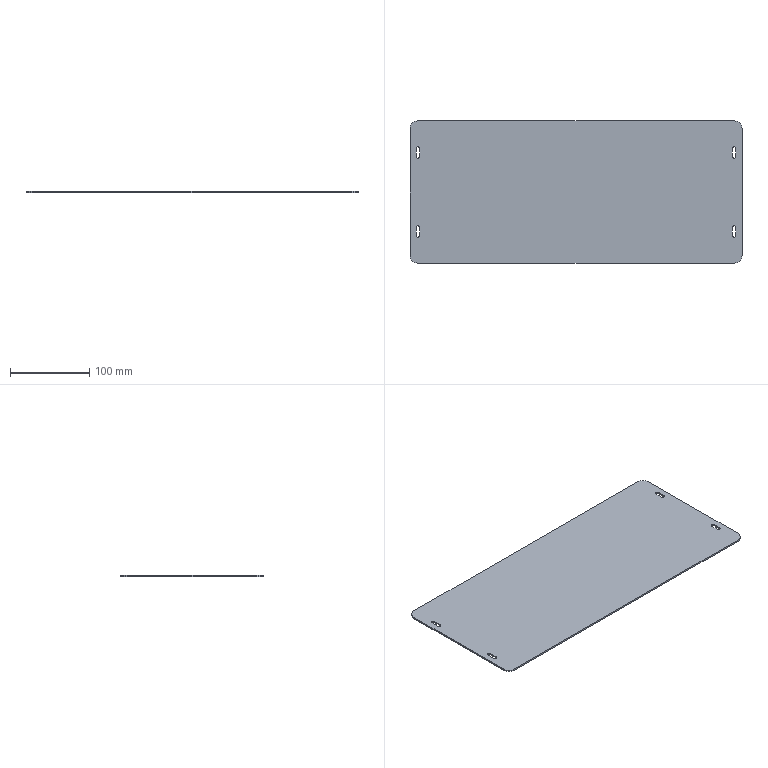Part | SolidWorks | features RefAxis 2, Extrusion 1, Fillet 1, HoleWzd 1, ICE 1 | 1 solid | 26 faces | box 420 x 180 x 2 mm | volume 150541 mm3 | plane 14 | cylinder 12 | commonest cylinder face diameters 4.5 x8 20 x4
STEP:
#1=CARTESIAN_POINT('',(210.,-80.,2.));
#2=VERTEX_POINT('',#1);
#3=CARTESIAN_POINT('',(210.,80.,2.));
#4=VERTEX_POINT('',#3);
#5=CARTESIAN_POINT('',(210.,90.,2.));
#6=DIRECTION('',(0.,1.,0.));
#7=VECTOR('',#6,1000.);
#8=LINE('',#5,#7);
#9=EDGE_CURVE('',#2,#4,#8,.T.);
#10=ORIENTED_EDGE('',*,*,#9,.F.);
#11=CARTESIAN_POINT('',(210.,-80.,0.));
#12=VERTEX_POINT('',#11);
#13=CARTESIAN_POINT('',(210.,-80.,2.));
#14=DIRECTION('',(0.,0.,-1.));
#15=VECTOR('',#14,1000.);
#16=LINE('',#13,#15);
#17=EDGE_CURVE('',#2,#12,#16,.T.);
#18=ORIENTED_EDGE('',*,*,#17,.T.);
#19=CARTESIAN_POINT('',(210.,80.,0.));
#20=VERTEX_POINT('',#19);
#21=CARTESIAN_POINT('',(210.,90.,0.));
#22=DIRECTION('',(0.,1.,0.));
#23=VECTOR('',#22,1000.);
#24=LINE('',#21,#23);
#25=EDGE_CURVE('',#12,#20,#24,.T.);
#26=ORIENTED_EDGE('',*,*,#25,.T.);
#27=CARTESIAN_POINT('',(210.,80.,2.));
#28=DIRECTION('',(0.,0.,1.));
#29=VECTOR('',#28,1000.);
#30=LINE('',#27,#29);
#31=EDGE_CURVE('',#20,#4,#30,.T.);
#32=ORIENTED_EDGE('',*,*,#31,.T.);
#33=EDGE_LOOP('',(#10,#18,#26,#32));
#34=FACE_OUTER_BOUND('',#33,.T.);
#35=CARTESIAN_POINT('',(210.,90.,2.));
#36=DIRECTION('',(-1.,0.,0.));
#37=DIRECTION('',(0.,0.,1.));
#38=AXIS2_PLACEMENT_3D('',#35,#36,#37);
#39=PLANE('',#38);
#40=ADVANCED_FACE('',(#34),#39,.F.);
#41=CARTESIAN_POINT('',(200.,90.,0.));
#42=VERTEX_POINT('',#41);
#43=CARTESIAN_POINT('',(-200.,90.,0.));
#44=VERTEX_POINT('',#43);
#45=CARTESIAN_POINT('',(-210.,90.,0.));
#46=DIRECTION('',(-1.,0.,0.));
#47=VECTOR('',#46,1000.);
#48=LINE('',#45,#47);
#49=EDGE_CURVE('',#42,#44,#48,.T.);
#50=ORIENTED_EDGE('',*,*,#49,.T.);
#51=CARTESIAN_POINT('',(-200.,90.,2.));
#52=VERTEX_POINT('',#51);
#53=CARTESIAN_POINT('',(-200.,90.,2.));
#54=DIRECTION('',(0.,0.,1.));
#55=VECTOR('',#54,1000.);
#56=LINE('',#53,#55);
#57=EDGE_CURVE('',#44,#52,#56,.T.);
#58=ORIENTED_EDGE('',*,*,#57,.T.);
#59=CARTESIAN_POINT('',(200.,90.,2.));
#60=VERTEX_POINT('',#59);
#61=CARTESIAN_POINT('',(-210.,90.,2.));
#62=DIRECTION('',(-1.,0.,0.));
#63=VECTOR('',#62,1000.);
#64=LINE('',#61,#63);
#65=EDGE_CURVE('',#60,#52,#64,.T.);
#66=ORIENTED_EDGE('',*,*,#65,.F.);
#67=CARTESIAN_POINT('',(200.,90.,2.));
#68=DIRECTION('',(0.,0.,-1.));
#69=VECTOR('',#68,1000.);
#70=LINE('',#67,#69);
#71=EDGE_CURVE('',#60,#42,#70,.T.);
#72=ORIENTED_EDGE('',*,*,#71,.T.);
#73=EDGE_LOOP('',(#50,#58,#66,#72));
#74=FACE_OUTER_BOUND('',#73,.T.);
#75=CARTESIAN_POINT('',(-210.,90.,2.));
#76=DIRECTION('',(0.,-1.,0.));
#77=DIRECTION('',(0.,0.,-1.));
#78=AXIS2_PLACEMENT_3D('',#75,#76,#77);
#79=PLANE('',#78);
#80=ADVANCED_FACE('',(#74),#79,.F.);
#81=CARTESIAN_POINT('',(-210.,80.,0.));
#82=VERTEX_POINT('',#81);
#83=CARTESIAN_POINT('',(-210.,-80.,0.));
#84=VERTEX_POINT('',#83);
#85=CARTESIAN_POINT('',(-210.,90.,0.));
#86=DIRECTION('',(0.,-1.,0.));
#87=VECTOR('',#86,1000.);
#88=LINE('',#85,#87);
#89=EDGE_CURVE('',#82,#84,#88,.T.);
#90=ORIENTED_EDGE('',*,*,#89,.T.);
#91=CARTESIAN_POINT('',(-210.,-80.,2.));
#92=VERTEX_POINT('',#91);
#93=CARTESIAN_POINT('',(-210.,-80.,2.));
#94=DIRECTION('',(0.,0.,1.));
#95=VECTOR('',#94,1000.);
#96=LINE('',#93,#95);
#97=EDGE_CURVE('',#84,#92,#96,.T.);
#98=ORIENTED_EDGE('',*,*,#97,.T.);
#99=CARTESIAN_POINT('',(-210.,80.,2.));
#100=VERTEX_POINT('',#99);
#101=CARTESIAN_POINT('',(-210.,90.,2.));
#102=DIRECTION('',(0.,-1.,0.));
#103=VECTOR('',#102,1000.);
#104=LINE('',#101,#103);
#105=EDGE_CURVE('',#100,#92,#104,.T.);
#106=ORIENTED_EDGE('',*,*,#105,.F.);
#107=CARTESIAN_POINT('',(-210.,80.,2.));
#108=DIRECTION('',(0.,0.,-1.));
#109=VECTOR('',#108,1000.);
#110=LINE('',#107,#109);
#111=EDGE_CURVE('',#100,#82,#110,.T.);
#112=ORIENTED_EDGE('',*,*,#111,.T.);
#113=EDGE_LOOP('',(#90,#98,#106,#112));
#114=FACE_OUTER_BOUND('',#113,.T.);
#115=CARTESIAN_POINT('',(-210.,90.,2.));
#116=DIRECTION('',(1.,0.,0.));
#117=DIRECTION('',(0.,0.,-1.));
#118=AXIS2_PLACEMENT_3D('',#115,#116,#117);
#119=PLANE('',#118);
#120=ADVANCED_FACE('',(#114),#119,.F.);
#121=CARTESIAN_POINT('',(-200.,-90.,2.));
#122=VERTEX_POINT('',#121);
#123=CARTESIAN_POINT('',(200.,-90.,2.));
#124=VERTEX_POINT('',#123);
#125=CARTESIAN_POINT('',(-210.,-90.,2.));
#126=DIRECTION('',(1.,0.,0.));
#127=VECTOR('',#126,1000.);
#128=LINE('',#125,#127);
#129=EDGE_CURVE('',#122,#124,#128,.T.);
#130=ORIENTED_EDGE('',*,*,#129,.F.);
#131=CARTESIAN_POINT('',(-200.,-90.,0.));
#132=VERTEX_POINT('',#131);
#133=CARTESIAN_POINT('',(-200.,-90.,2.));
#134=DIRECTION('',(0.,0.,-1.));
#135=VECTOR('',#134,1000.);
#136=LINE('',#133,#135);
#137=EDGE_CURVE('',#122,#132,#136,.T.);
#138=ORIENTED_EDGE('',*,*,#137,.T.);
#139=CARTESIAN_POINT('',(200.,-90.,0.));
#140=VERTEX_POINT('',#139);
#141=CARTESIAN_POINT('',(-210.,-90.,0.));
#142=DIRECTION('',(1.,0.,0.));
#143=VECTOR('',#142,1000.);
#144=LINE('',#141,#143);
#145=EDGE_CURVE('',#132,#140,#144,.T.);
#146=ORIENTED_EDGE('',*,*,#145,.T.);
#147=CARTESIAN_POINT('',(200.,-90.,2.));
#148=DIRECTION('',(0.,0.,1.));
#149=VECTOR('',#148,1000.);
#150=LINE('',#147,#149);
#151=EDGE_CURVE('',#140,#124,#150,.T.);
#152=ORIENTED_EDGE('',*,*,#151,.T.);
#153=EDGE_LOOP('',(#130,#138,#146,#152));
#154=FACE_OUTER_BOUND('',#153,.T.);
#155=CARTESIAN_POINT('',(-210.,-90.,2.));
#156=DIRECTION('',(0.,1.,0.));
#157=DIRECTION('',(0.,0.,1.));
#158=AXIS2_PLACEMENT_3D('',#155,#156,#157);
#159=PLANE('',#158);
#160=ADVANCED_FACE('',(#154),#159,.F.);
#161=CARTESIAN_POINT('',(-197.75,55.,2.));
#162=VERTEX_POINT('',#161);
#163=CARTESIAN_POINT('',(-202.25,55.,2.));
#164=VERTEX_POINT('',#163);
#165=CARTESIAN_POINT('',(-200.,55.,2.));
#166=DIRECTION('',(0.,0.,1.));
#167=DIRECTION('',(-1.,0.,0.));
#168=AXIS2_PLACEMENT_3D('',#165,#166,#167);
#169=CIRCLE('',#168,2.25);
#170=EDGE_CURVE('',#162,#164,#169,.T.);
#171=ORIENTED_EDGE('',*,*,#170,.F.);
#172=CARTESIAN_POINT('',(-197.75,45.,2.));
#173=VERTEX_POINT('',#172);
#174=CARTESIAN_POINT('',(-197.75,55.,2.));
#175=DIRECTION('',(0.,1.,0.));
#176=VECTOR('',#175,1000.);
#177=LINE('',#174,#176);
#178=EDGE_CURVE('',#173,#162,#177,.T.);
#179=ORIENTED_EDGE('',*,*,#178,.F.);
#180=CARTESIAN_POINT('',(-202.25,45.,2.));
#181=VERTEX_POINT('',#180);
#182=CARTESIAN_POINT('',(-200.,45.,2.));
#183=DIRECTION('',(0.,0.,1.));
#184=DIRECTION('',(-1.,0.,0.));
#185=AXIS2_PLACEMENT_3D('',#182,#183,#184);
#186=CIRCLE('',#185,2.25);
#187=EDGE_CURVE('',#181,#173,#186,.T.);
#188=ORIENTED_EDGE('',*,*,#187,.F.);
#189=CARTESIAN_POINT('',(-202.25,55.,2.));
#190=DIRECTION('',(0.,-1.,0.));
#191=VECTOR('',#190,1000.);
#192=LINE('',#189,#191);
#193=EDGE_CURVE('',#164,#181,#192,.T.);
#194=ORIENTED_EDGE('',*,*,#193,.F.);
#195=EDGE_LOOP('',(#171,#179,#188,#194));
#196=FACE_BOUND('',#195,.T.);
#197=CARTESIAN_POINT('',(-202.25,-55.,2.));
#198=VERTEX_POINT('',#197);
#199=CARTESIAN_POINT('',(-197.75,-55.,2.));
#200=VERTEX_POINT('',#199);
#201=CARTESIAN_POINT('',(-200.,-55.,2.));
#202=DIRECTION('',(0.,0.,1.));
#203=DIRECTION('',(-1.,0.,0.));
#204=AXIS2_PLACEMENT_3D('',#201,#202,#203);
#205=CIRCLE('',#204,2.25);
#206=EDGE_CURVE('',#198,#200,#205,.T.);
#207=ORIENTED_EDGE('',*,*,#206,.F.);
#208=CARTESIAN_POINT('',(-202.25,-45.,2.));
#209=VERTEX_POINT('',#208);
#210=CARTESIAN_POINT('',(-202.25,-55.,2.));
#211=DIRECTION('',(0.,-1.,0.));
#212=VECTOR('',#211,1000.);
#213=LINE('',#210,#212);
#214=EDGE_CURVE('',#209,#198,#213,.T.);
#215=ORIENTED_EDGE('',*,*,#214,.F.);
#216=CARTESIAN_POINT('',(-197.75,-45.,2.));
#217=VERTEX_POINT('',#216);
#218=CARTESIAN_POINT('',(-200.,-45.,2.));
#219=DIRECTION('',(0.,0.,1.));
#220=DIRECTION('',(-1.,0.,0.));
#221=AXIS2_PLACEMENT_3D('',#218,#219,#220);
#222=CIRCLE('',#221,2.25);
#223=EDGE_CURVE('',#217,#209,#222,.T.);
#224=ORIENTED_EDGE('',*,*,#223,.F.);
#225=CARTESIAN_POINT('',(-197.75,-55.,2.));
#226=DIRECTION('',(0.,1.,0.));
#227=VECTOR('',#226,1000.);
#228=LINE('',#225,#227);
#229=EDGE_CURVE('',#200,#217,#228,.T.);
#230=ORIENTED_EDGE('',*,*,#229,.F.);
#231=EDGE_LOOP('',(#207,#215,#224,#230));
#232=FACE_BOUND('',#231,.T.);
#233=CARTESIAN_POINT('',(197.75,-55.,2.));
#234=VERTEX_POINT('',#233);
#235=CARTESIAN_POINT('',(202.25,-55.,2.));
#236=VERTEX_POINT('',#235);
#237=CARTESIAN_POINT('',(200.,-55.,2.));
#238=DIRECTION('',(0.,0.,1.));
#239=DIRECTION('',(1.,0.,0.));
#240=AXIS2_PLACEMENT_3D('',#237,#238,#239);
#241=CIRCLE('',#240,2.25);
#242=EDGE_CURVE('',#234,#236,#241,.T.);
#243=ORIENTED_EDGE('',*,*,#242,.F.);
#244=CARTESIAN_POINT('',(197.75,-45.,2.));
#245=VERTEX_POINT('',#244);
#246=CARTESIAN_POINT('',(197.75,-55.,2.));
#247=DIRECTION('',(0.,-1.,0.));
#248=VECTOR('',#247,1000.);
#249=LINE('',#246,#248);
#250=EDGE_CURVE('',#245,#234,#249,.T.);
#251=ORIENTED_EDGE('',*,*,#250,.F.);
#252=CARTESIAN_POINT('',(202.25,-45.,2.));
#253=VERTEX_POINT('',#252);
#254=CARTESIAN_POINT('',(200.,-45.,2.));
#255=DIRECTION('',(0.,0.,1.));
#256=DIRECTION('',(1.,0.,0.));
#257=AXIS2_PLACEMENT_3D('',#254,#255,#256);
#258=CIRCLE('',#257,2.25);
#259=EDGE_CURVE('',#253,#245,#258,.T.);
#260=ORIENTED_EDGE('',*,*,#259,.F.);
#261=CARTESIAN_POINT('',(202.25,-55.,2.));
#262=DIRECTION('',(0.,1.,0.));
#263=VECTOR('',#262,1000.);
#264=LINE('',#261,#263);
#265=EDGE_CURVE('',#236,#253,#264,.T.);
#266=ORIENTED_EDGE('',*,*,#265,.F.);
#267=EDGE_LOOP('',(#243,#251,#260,#266));
#268=FACE_BOUND('',#267,.T.);
#269=CARTESIAN_POINT('',(202.25,55.,2.));
#270=VERTEX_POINT('',#269);
#271=CARTESIAN_POINT('',(197.75,55.,2.));
#272=VERTEX_POINT('',#271);
#273=CARTESIAN_POINT('',(200.,55.,2.));
#274=DIRECTION('',(0.,0.,1.));
#275=DIRECTION('',(1.,0.,0.));
#276=AXIS2_PLACEMENT_3D('',#273,#274,#275);
#277=CIRCLE('',#276,2.25);
#278=EDGE_CURVE('',#270,#272,#277,.T.);
#279=ORIENTED_EDGE('',*,*,#278,.F.);
#280=CARTESIAN_POINT('',(202.25,45.,2.));
#281=VERTEX_POINT('',#280);
#282=CARTESIAN_POINT('',(202.25,55.,2.));
#283=DIRECTION('',(0.,1.,0.));
#284=VECTOR('',#283,1000.);
#285=LINE('',#282,#284);
#286=EDGE_CURVE('',#281,#270,#285,.T.);
#287=ORIENTED_EDGE('',*,*,#286,.F.);
#288=CARTESIAN_POINT('',(197.75,45.,2.));
#289=VERTEX_POINT('',#288);
#290=CARTESIAN_POINT('',(200.,45.,2.));
#291=DIRECTION('',(0.,0.,1.));
#292=DIRECTION('',(1.,0.,0.));
#293=AXIS2_PLACEMENT_3D('',#290,#291,#292);
#294=CIRCLE('',#293,2.25);
#295=EDGE_CURVE('',#289,#281,#294,.T.);
#296=ORIENTED_EDGE('',*,*,#295,.F.);
#297=CARTESIAN_POINT('',(197.75,55.,2.));
#298=DIRECTION('',(0.,-1.,0.));
#299=VECTOR('',#298,1000.);
#300=LINE('',#297,#299);
#301=EDGE_CURVE('',#272,#289,#300,.T.);
#302=ORIENTED_EDGE('',*,*,#301,.F.);
#303=EDGE_LOOP('',(#279,#287,#296,#302));
#304=FACE_BOUND('',#303,.T.);
#305=ORIENTED_EDGE('',*,*,#105,.T.);
#306=CARTESIAN_POINT('',(-200.,-80.,2.));
#307=DIRECTION('',(0.,0.,1.));
#308=DIRECTION('',(1.,0.,0.));
#309=AXIS2_PLACEMENT_3D('',#306,#307,#308);
#310=CIRCLE('',#309,10.);
#311=EDGE_CURVE('',#92,#122,#310,.T.);
#312=ORIENTED_EDGE('',*,*,#311,.T.);
#313=ORIENTED_EDGE('',*,*,#129,.T.);
#314=CARTESIAN_POINT('',(200.,-80.,2.));
#315=DIRECTION('',(0.,0.,1.));
#316=DIRECTION('',(1.,0.,0.));
#317=AXIS2_PLACEMENT_3D('',#314,#315,#316);
#318=CIRCLE('',#317,10.);
#319=EDGE_CURVE('',#124,#2,#318,.T.);
#320=ORIENTED_EDGE('',*,*,#319,.T.);
#321=ORIENTED_EDGE('',*,*,#9,.T.);
#322=CARTESIAN_POINT('',(200.,80.,2.));
#323=DIRECTION('',(0.,0.,1.));
#324=DIRECTION('',(1.,0.,0.));
#325=AXIS2_PLACEMENT_3D('',#322,#323,#324);
#326=CIRCLE('',#325,10.);
#327=EDGE_CURVE('',#4,#60,#326,.T.);
#328=ORIENTED_EDGE('',*,*,#327,.T.);
#329=ORIENTED_EDGE('',*,*,#65,.T.);
#330=CARTESIAN_POINT('',(-200.,80.,2.));
#331=DIRECTION('',(0.,0.,1.));
#332=DIRECTION('',(1.,0.,0.));
#333=AXIS2_PLACEMENT_3D('',#330,#331,#332);
#334=CIRCLE('',#333,10.);
#335=EDGE_CURVE('',#52,#100,#334,.T.);
#336=ORIENTED_EDGE('',*,*,#335,.T.);
#337=EDGE_LOOP('',(#305,#312,#313,#320,#321,#328,#329,#336));
#338=FACE_OUTER_BOUND('',#337,.T.);
#339=CARTESIAN_POINT('',(0.,0.,2.));
#340=DIRECTION('',(0.,0.,1.));
#341=DIRECTION('',(1.,0.,0.));
#342=AXIS2_PLACEMENT_3D('',#339,#340,#341);
#343=PLANE('',#342);
#344=ADVANCED_FACE('',(#196,#232,#268,#304,#338),#343,.T.);
#345=CARTESIAN_POINT('',(-197.75,45.,0.));
#346=VERTEX_POINT('',#345);
#347=CARTESIAN_POINT('',(-197.75,55.,0.));
#348=VERTEX_POINT('',#347);
#349=CARTESIAN_POINT('',(-197.75,0.,0.));
#350=DIRECTION('',(0.,1.,0.));
#351=VECTOR('',#350,1000.);
#352=LINE('',#349,#351);
#353=EDGE_CURVE('',#346,#348,#352,.T.);
#354=ORIENTED_EDGE('',*,*,#353,.T.);
#355=CARTESIAN_POINT('',(-202.25,55.,0.));
#356=VERTEX_POINT('',#355);
#357=CARTESIAN_POINT('',(-200.,55.,0.));
#358=DIRECTION('',(0.,0.,1.));
#359=DIRECTION('',(1.,0.,0.));
#360=AXIS2_PLACEMENT_3D('',#357,#358,#359);
#361=CIRCLE('',#360,2.25);
#362=EDGE_CURVE('',#348,#356,#361,.T.);
#363=ORIENTED_EDGE('',*,*,#362,.T.);
#364=CARTESIAN_POINT('',(-202.25,45.,0.));
#365=VERTEX_POINT('',#364);
#366=CARTESIAN_POINT('',(-202.25,0.,0.));
#367=DIRECTION('',(0.,-1.,0.));
#368=VECTOR('',#367,1000.);
#369=LINE('',#366,#368);
#370=EDGE_CURVE('',#356,#365,#369,.T.);
#371=ORIENTED_EDGE('',*,*,#370,.T.);
#372=CARTESIAN_POINT('',(-200.,45.,0.));
#373=DIRECTION('',(0.,0.,1.));
#374=DIRECTION('',(1.,0.,0.));
#375=AXIS2_PLACEMENT_3D('',#372,#373,#374);
#376=CIRCLE('',#375,2.25);
#377=EDGE_CURVE('',#365,#346,#376,.T.);
#378=ORIENTED_EDGE('',*,*,#377,.T.);
#379=EDGE_LOOP('',(#354,#363,#371,#378));
#380=FACE_BOUND('',#379,.T.);
#381=CARTESIAN_POINT('',(-202.25,-45.,0.));
#382=VERTEX_POINT('',#381);
#383=CARTESIAN_POINT('',(-202.25,-55.,0.));
#384=VERTEX_POINT('',#383);
#385=CARTESIAN_POINT('',(-202.25,0.,0.));
#386=DIRECTION('',(0.,-1.,0.));
#387=VECTOR('',#386,1000.);
#388=LINE('',#385,#387);
#389=EDGE_CURVE('',#382,#384,#388,.T.);
#390=ORIENTED_EDGE('',*,*,#389,.T.);
#391=CARTESIAN_POINT('',(-197.75,-55.,0.));
#392=VERTEX_POINT('',#391);
#393=CARTESIAN_POINT('',(-200.,-55.,0.));
#394=DIRECTION('',(0.,0.,1.));
#395=DIRECTION('',(1.,0.,0.));
#396=AXIS2_PLACEMENT_3D('',#393,#394,#395);
#397=CIRCLE('',#396,2.25);
#398=EDGE_CURVE('',#384,#392,#397,.T.);
#399=ORIENTED_EDGE('',*,*,#398,.T.);
#400=CARTESIAN_POINT('',(-197.75,-45.,0.));
#401=VERTEX_POINT('',#400);
#402=CARTESIAN_POINT('',(-197.75,0.,0.));
#403=DIRECTION('',(0.,1.,0.));
#404=VECTOR('',#403,1000.);
#405=LINE('',#402,#404);
#406=EDGE_CURVE('',#392,#401,#405,.T.);
#407=ORIENTED_EDGE('',*,*,#406,.T.);
#408=CARTESIAN_POINT('',(-200.,-45.,0.));
#409=DIRECTION('',(0.,0.,1.));
#410=DIRECTION('',(1.,0.,0.));
#411=AXIS2_PLACEMENT_3D('',#408,#409,#410);
#412=CIRCLE('',#411,2.25);
#413=EDGE_CURVE('',#401,#382,#412,.T.);
#414=ORIENTED_EDGE('',*,*,#413,.T.);
#415=EDGE_LOOP('',(#390,#399,#407,#414));
#416=FACE_BOUND('',#415,.T.);
#417=CARTESIAN_POINT('',(197.75,-45.,0.));
#418=VERTEX_POINT('',#417);
#419=CARTESIAN_POINT('',(197.75,-55.,0.));
#420=VERTEX_POINT('',#419);
#421=CARTESIAN_POINT('',(197.75,0.,0.));
#422=DIRECTION('',(0.,-1.,0.));
#423=VECTOR('',#422,1000.);
#424=LINE('',#421,#423);
#425=EDGE_CURVE('',#418,#420,#424,.T.);
#426=ORIENTED_EDGE('',*,*,#425,.T.);
#427=CARTESIAN_POINT('',(202.25,-55.,0.));
#428=VERTEX_POINT('',#427);
#429=CARTESIAN_POINT('',(200.,-55.,0.));
#430=DIRECTION('',(0.,0.,1.));
#431=DIRECTION('',(1.,0.,0.));
#432=AXIS2_PLACEMENT_3D('',#429,#430,#431);
#433=CIRCLE('',#432,2.25);
#434=EDGE_CURVE('',#420,#428,#433,.T.);
#435=ORIENTED_EDGE('',*,*,#434,.T.);
#436=CARTESIAN_POINT('',(202.25,-45.,0.));
#437=VERTEX_POINT('',#436);
#438=CARTESIAN_POINT('',(202.25,0.,0.));
#439=DIRECTION('',(0.,1.,0.));
#440=VECTOR('',#439,1000.);
#441=LINE('',#438,#440);
#442=EDGE_CURVE('',#428,#437,#441,.T.);
#443=ORIENTED_EDGE('',*,*,#442,.T.);
#444=CARTESIAN_POINT('',(200.,-45.,0.));
#445=DIRECTION('',(0.,0.,1.));
#446=DIRECTION('',(1.,0.,0.));
#447=AXIS2_PLACEMENT_3D('',#444,#445,#446);
#448=CIRCLE('',#447,2.25);
#449=EDGE_CURVE('',#437,#418,#448,.T.);
#450=ORIENTED_EDGE('',*,*,#449,.T.);
#451=EDGE_LOOP('',(#426,#435,#443,#450));
#452=FACE_BOUND('',#451,.T.);
#453=CARTESIAN_POINT('',(202.25,45.,0.));
#454=VERTEX_POINT('',#453);
#455=CARTESIAN_POINT('',(202.25,55.,0.));
#456=VERTEX_POINT('',#455);
#457=CARTESIAN_POINT('',(202.25,0.,0.));
#458=DIRECTION('',(0.,1.,0.));
#459=VECTOR('',#458,1000.);
#460=LINE('',#457,#459);
#461=EDGE_CURVE('',#454,#456,#460,.T.);
#462=ORIENTED_EDGE('',*,*,#461,.T.);
#463=CARTESIAN_POINT('',(197.75,55.,0.));
#464=VERTEX_POINT('',#463);
#465=CARTESIAN_POINT('',(200.,55.,0.));
#466=DIRECTION('',(0.,0.,1.));
#467=DIRECTION('',(1.,0.,0.));
#468=AXIS2_PLACEMENT_3D('',#465,#466,#467);
#469=CIRCLE('',#468,2.25);
#470=EDGE_CURVE('',#456,#464,#469,.T.);
#471=ORIENTED_EDGE('',*,*,#470,.T.);
#472=CARTESIAN_POINT('',(197.75,45.,0.));
#473=VERTEX_POINT('',#472);
#474=CARTESIAN_POINT('',(197.75,0.,0.));
#475=DIRECTION('',(0.,-1.,0.));
#476=VECTOR('',#475,1000.);
#477=LINE('',#474,#476);
#478=EDGE_CURVE('',#464,#473,#477,.T.);
#479=ORIENTED_EDGE('',*,*,#478,.T.);
#480=CARTESIAN_POINT('',(200.,45.,0.));
#481=DIRECTION('',(0.,0.,1.));
#482=DIRECTION('',(1.,0.,0.));
#483=AXIS2_PLACEMENT_3D('',#480,#481,#482);
#484=CIRCLE('',#483,2.25);
#485=EDGE_CURVE('',#473,#454,#484,.T.);
#486=ORIENTED_EDGE('',*,*,#485,.T.);
#487=EDGE_LOOP('',(#462,#471,#479,#486));
#488=FACE_BOUND('',#487,.T.);
#489=ORIENTED_EDGE('',*,*,#145,.F.);
#490=CARTESIAN_POINT('',(-200.,-80.,0.));
#491=DIRECTION('',(0.,0.,-1.));
#492=DIRECTION('',(1.,0.,0.));
#493=AXIS2_PLACEMENT_3D('',#490,#491,#492);
#494=CIRCLE('',#493,10.);
#495=EDGE_CURVE('',#132,#84,#494,.T.);
#496=ORIENTED_EDGE('',*,*,#495,.T.);
#497=ORIENTED_EDGE('',*,*,#89,.F.);
#498=CARTESIAN_POINT('',(-200.,80.,0.));
#499=DIRECTION('',(0.,0.,-1.));
#500=DIRECTION('',(1.,0.,0.));
#501=AXIS2_PLACEMENT_3D('',#498,#499,#500);
#502=CIRCLE('',#501,10.);
#503=EDGE_CURVE('',#82,#44,#502,.T.);
#504=ORIENTED_EDGE('',*,*,#503,.T.);
#505=ORIENTED_EDGE('',*,*,#49,.F.);
#506=CARTESIAN_POINT('',(200.,80.,0.));
#507=DIRECTION('',(0.,0.,-1.));
#508=DIRECTION('',(1.,0.,0.));
#509=AXIS2_PLACEMENT_3D('',#506,#507,#508);
#510=CIRCLE('',#509,10.);
#511=EDGE_CURVE('',#42,#20,#510,.T.);
#512=ORIENTED_EDGE('',*,*,#511,.T.);
#513=ORIENTED_EDGE('',*,*,#25,.F.);
#514=CARTESIAN_POINT('',(200.,-80.,0.));
#515=DIRECTION('',(0.,0.,-1.));
#516=DIRECTION('',(1.,0.,0.));
#517=AXIS2_PLACEMENT_3D('',#514,#515,#516);
#518=CIRCLE('',#517,10.);
#519=EDGE_CURVE('',#12,#140,#518,.T.);
#520=ORIENTED_EDGE('',*,*,#519,.T.);
#521=EDGE_LOOP('',(#489,#496,#497,#504,#505,#512,#513,#520));
#522=FACE_OUTER_BOUND('',#521,.T.);
#523=CARTESIAN_POINT('',(0.,0.,0.));
#524=DIRECTION('',(0.,0.,1.));
#525=DIRECTION('',(1.,0.,0.));
#526=AXIS2_PLACEMENT_3D('',#523,#524,#525);
#527=PLANE('',#526);
#528=ADVANCED_FACE('',(#380,#416,#452,#488,#522),#527,.F.);
#529=CARTESIAN_POINT('',(202.25,55.,-8.));
#530=DIRECTION('',(0.,0.,1.));
#531=VECTOR('',#530,1000.);
#532=LINE('',#529,#531);
#533=EDGE_CURVE('',#456,#270,#532,.T.);
#534=ORIENTED_EDGE('',*,*,#533,.T.);
#535=ORIENTED_EDGE('',*,*,#278,.T.);
#536=CARTESIAN_POINT('',(197.75,55.,-8.));
#537=DIRECTION('',(0.,0.,1.));
#538=VECTOR('',#537,1000.);
#539=LINE('',#536,#538);
#540=EDGE_CURVE('',#464,#272,#539,.T.);
#541=ORIENTED_EDGE('',*,*,#540,.F.);
#542=ORIENTED_EDGE('',*,*,#470,.F.);
#543=EDGE_LOOP('',(#534,#535,#541,#542));
#544=FACE_OUTER_BOUND('',#543,.T.);
#545=CARTESIAN_POINT('',(200.,55.,-8.));
#546=DIRECTION('',(0.,0.,1.));
#547=DIRECTION('',(1.,0.,0.));
#548=AXIS2_PLACEMENT_3D('',#545,#546,#547);
#549=CYLINDRICAL_SURFACE('',#548,2.25);
#550=ADVANCED_FACE('',(#544),#549,.F.);
#551=CARTESIAN_POINT('',(202.25,45.,-8.));
#552=DIRECTION('',(0.,0.,1.));
#553=VECTOR('',#552,1000.);
#554=LINE('',#551,#553);
#555=EDGE_CURVE('',#454,#281,#554,.T.);
#556=ORIENTED_EDGE('',*,*,#555,.T.);
#557=ORIENTED_EDGE('',*,*,#286,.T.);
#558=ORIENTED_EDGE('',*,*,#533,.F.);
#559=ORIENTED_EDGE('',*,*,#461,.F.);
#560=EDGE_LOOP('',(#556,#557,#558,#559));
#561=FACE_OUTER_BOUND('',#560,.T.);
#562=CARTESIAN_POINT('',(202.25,55.,-8.));
#563=DIRECTION('',(1.,0.,0.));
#564=DIRECTION('',(0.,0.,-1.));
#565=AXIS2_PLACEMENT_3D('',#562,#563,#564);
#566=PLANE('',#565);
#567=ADVANCED_FACE('',(#561),#566,.F.);
#568=CARTESIAN_POINT('',(197.75,45.,-8.));
#569=DIRECTION('',(0.,0.,1.));
#570=VECTOR('',#569,1000.);
#571=LINE('',#568,#570);
#572=EDGE_CURVE('',#473,#289,#571,.T.);
#573=ORIENTED_EDGE('',*,*,#572,.T.);
#574=ORIENTED_EDGE('',*,*,#295,.T.);
#575=ORIENTED_EDGE('',*,*,#555,.F.);
#576=ORIENTED_EDGE('',*,*,#485,.F.);
#577=EDGE_LOOP('',(#573,#574,#575,#576));
#578=FACE_OUTER_BOUND('',#577,.T.);
#579=CARTESIAN_POINT('',(200.,45.,-8.));
#580=DIRECTION('',(0.,0.,1.));
#581=DIRECTION('',(1.,0.,0.));
#582=AXIS2_PLACEMENT_3D('',#579,#580,#581);
#583=CYLINDRICAL_SURFACE('',#582,2.25);
#584=ADVANCED_FACE('',(#578),#583,.F.);
#585=ORIENTED_EDGE('',*,*,#540,.T.);
#586=ORIENTED_EDGE('',*,*,#301,.T.);
#587=ORIENTED_EDGE('',*,*,#572,.F.);
#588=ORIENTED_EDGE('',*,*,#478,.F.);
#589=EDGE_LOOP('',(#585,#586,#587,#588));
#590=FACE_OUTER_BOUND('',#589,.T.);
#591=CARTESIAN_POINT('',(197.75,55.,-8.));
#592=DIRECTION('',(-1.,0.,0.));
#593=DIRECTION('',(0.,0.,1.));
#594=AXIS2_PLACEMENT_3D('',#591,#592,#593);
#595=PLANE('',#594);
#596=ADVANCED_FACE('',(#590),#595,.F.);
#597=CARTESIAN_POINT('',(197.75,-55.,-8.));
#598=DIRECTION('',(0.,0.,1.));
#599=VECTOR('',#598,1000.);
#600=LINE('',#597,#599);
#601=EDGE_CURVE('',#420,#234,#600,.T.);
#602=ORIENTED_EDGE('',*,*,#601,.T.);
#603=ORIENTED_EDGE('',*,*,#242,.T.);
#604=CARTESIAN_POINT('',(202.25,-55.,-8.));
#605=DIRECTION('',(0.,0.,1.));
#606=VECTOR('',#605,1000.);
#607=LINE('',#604,#606);
#608=EDGE_CURVE('',#428,#236,#607,.T.);
#609=ORIENTED_EDGE('',*,*,#608,.F.);
#610=ORIENTED_EDGE('',*,*,#434,.F.);
#611=EDGE_LOOP('',(#602,#603,#609,#610));
#612=FACE_OUTER_BOUND('',#611,.T.);
#613=CARTESIAN_POINT('',(200.,-55.,-8.));
#614=DIRECTION('',(0.,0.,1.));
#615=DIRECTION('',(1.,0.,0.));
#616=AXIS2_PLACEMENT_3D('',#613,#614,#615);
#617=CYLINDRICAL_SURFACE('',#616,2.25);
#618=ADVANCED_FACE('',(#612),#617,.F.);
#619=CARTESIAN_POINT('',(197.75,-45.,-8.));
#620=DIRECTION('',(0.,0.,1.));
#621=VECTOR('',#620,1000.);
#622=LINE('',#619,#621);
#623=EDGE_CURVE('',#418,#245,#622,.T.);
#624=ORIENTED_EDGE('',*,*,#623,.T.);
#625=ORIENTED_EDGE('',*,*,#250,.T.);
#626=ORIENTED_EDGE('',*,*,#601,.F.);
#627=ORIENTED_EDGE('',*,*,#425,.F.);
#628=EDGE_LOOP('',(#624,#625,#626,#627));
#629=FACE_OUTER_BOUND('',#628,.T.);
#630=CARTESIAN_POINT('',(197.75,-55.,-8.));
#631=DIRECTION('',(-1.,0.,0.));
#632=DIRECTION('',(0.,0.,1.));
#633=AXIS2_PLACEMENT_3D('',#630,#631,#632);
#634=PLANE('',#633);
#635=ADVANCED_FACE('',(#629),#634,.F.);
#636=CARTESIAN_POINT('',(202.25,-45.,-8.));
#637=DIRECTION('',(0.,0.,1.));
#638=VECTOR('',#637,1000.);
#639=LINE('',#636,#638);
#640=EDGE_CURVE('',#437,#253,#639,.T.);
#641=ORIENTED_EDGE('',*,*,#640,.T.);
#642=ORIENTED_EDGE('',*,*,#259,.T.);
#643=ORIENTED_EDGE('',*,*,#623,.F.);
#644=ORIENTED_EDGE('',*,*,#449,.F.);
#645=EDGE_LOOP('',(#641,#642,#643,#644));
#646=FACE_OUTER_BOUND('',#645,.T.);
#647=CARTESIAN_POINT('',(200.,-45.,-8.));
#648=DIRECTION('',(0.,0.,1.));
#649=DIRECTION('',(1.,0.,0.));
#650=AXIS2_PLACEMENT_3D('',#647,#648,#649);
#651=CYLINDRICAL_SURFACE('',#650,2.25);
#652=ADVANCED_FACE('',(#646),#651,.F.);
#653=ORIENTED_EDGE('',*,*,#608,.T.);
#654=ORIENTED_EDGE('',*,*,#265,.T.);
#655=ORIENTED_EDGE('',*,*,#640,.F.);
#656=ORIENTED_EDGE('',*,*,#442,.F.);
#657=EDGE_LOOP('',(#653,#654,#655,#656));
#658=FACE_OUTER_BOUND('',#657,.T.);
#659=CARTESIAN_POINT('',(202.25,-55.,-8.));
#660=DIRECTION('',(1.,0.,0.));
#661=DIRECTION('',(0.,0.,-1.));
#662=AXIS2_PLACEMENT_3D('',#659,#660,#661);
#663=PLANE('',#662);
#664=ADVANCED_FACE('',(#658),#663,.F.);
#665=CARTESIAN_POINT('',(-202.25,-55.,-8.));
#666=DIRECTION('',(0.,0.,1.));
#667=VECTOR('',#666,1000.);
#668=LINE('',#665,#667);
#669=EDGE_CURVE('',#384,#198,#668,.T.);
#670=ORIENTED_EDGE('',*,*,#669,.T.);
#671=ORIENTED_EDGE('',*,*,#206,.T.);
#672=CARTESIAN_POINT('',(-197.75,-55.,-8.));
#673=DIRECTION('',(0.,0.,1.));
#674=VECTOR('',#673,1000.);
#675=LINE('',#672,#674);
#676=EDGE_CURVE('',#392,#200,#675,.T.);
#677=ORIENTED_EDGE('',*,*,#676,.F.);
#678=ORIENTED_EDGE('',*,*,#398,.F.);
#679=EDGE_LOOP('',(#670,#671,#677,#678));
#680=FACE_OUTER_BOUND('',#679,.T.);
#681=CARTESIAN_POINT('',(-200.,-55.,-8.));
#682=DIRECTION('',(0.,0.,1.));
#683=DIRECTION('',(1.,0.,0.));
#684=AXIS2_PLACEMENT_3D('',#681,#682,#683);
#685=CYLINDRICAL_SURFACE('',#684,2.25);
#686=ADVANCED_FACE('',(#680),#685,.F.);
#687=CARTESIAN_POINT('',(-202.25,-45.,-8.));
#688=DIRECTION('',(0.,0.,1.));
#689=VECTOR('',#688,1000.);
#690=LINE('',#687,#689);
#691=EDGE_CURVE('',#382,#209,#690,.T.);
#692=ORIENTED_EDGE('',*,*,#691,.T.);
#693=ORIENTED_EDGE('',*,*,#214,.T.);
#694=ORIENTED_EDGE('',*,*,#669,.F.);
#695=ORIENTED_EDGE('',*,*,#389,.F.);
#696=EDGE_LOOP('',(#692,#693,#694,#695));
#697=FACE_OUTER_BOUND('',#696,.T.);
#698=CARTESIAN_POINT('',(-202.25,-55.,-8.));
#699=DIRECTION('',(-1.,0.,0.));
#700=DIRECTION('',(0.,0.,1.));
#701=AXIS2_PLACEMENT_3D('',#698,#699,#700);
#702=PLANE('',#701);
#703=ADVANCED_FACE('',(#697),#702,.F.);
#704=CARTESIAN_POINT('',(-197.75,-45.,-8.));
#705=DIRECTION('',(0.,0.,1.));
#706=VECTOR('',#705,1000.);
#707=LINE('',#704,#706);
#708=EDGE_CURVE('',#401,#217,#707,.T.);
#709=ORIENTED_EDGE('',*,*,#708,.T.);
#710=ORIENTED_EDGE('',*,*,#223,.T.);
#711=ORIENTED_EDGE('',*,*,#691,.F.);
#712=ORIENTED_EDGE('',*,*,#413,.F.);
#713=EDGE_LOOP('',(#709,#710,#711,#712));
#714=FACE_OUTER_BOUND('',#713,.T.);
#715=CARTESIAN_POINT('',(-200.,-45.,-8.));
#716=DIRECTION('',(0.,0.,1.));
#717=DIRECTION('',(1.,0.,0.));
#718=AXIS2_PLACEMENT_3D('',#715,#716,#717);
#719=CYLINDRICAL_SURFACE('',#718,2.25);
#720=ADVANCED_FACE('',(#714),#719,.F.);
#721=ORIENTED_EDGE('',*,*,#676,.T.);
#722=ORIENTED_EDGE('',*,*,#229,.T.);
#723=ORIENTED_EDGE('',*,*,#708,.F.);
#724=ORIENTED_EDGE('',*,*,#406,.F.);
#725=EDGE_LOOP('',(#721,#722,#723,#724));
#726=FACE_OUTER_BOUND('',#725,.T.);
#727=CARTESIAN_POINT('',(-197.75,-55.,-8.));
#728=DIRECTION('',(1.,0.,0.));
#729=DIRECTION('',(0.,0.,-1.));
#730=AXIS2_PLACEMENT_3D('',#727,#728,#729);
#731=PLANE('',#730);
#732=ADVANCED_FACE('',(#726),#731,.F.);
#733=CARTESIAN_POINT('',(-197.75,55.,-8.));
#734=DIRECTION('',(0.,0.,1.));
#735=VECTOR('',#734,1000.);
#736=LINE('',#733,#735);
#737=EDGE_CURVE('',#348,#162,#736,.T.);
#738=ORIENTED_EDGE('',*,*,#737,.T.);
#739=ORIENTED_EDGE('',*,*,#170,.T.);
#740=CARTESIAN_POINT('',(-202.25,55.,-8.));
#741=DIRECTION('',(0.,0.,1.));
#742=VECTOR('',#741,1000.);
#743=LINE('',#740,#742);
#744=EDGE_CURVE('',#356,#164,#743,.T.);
#745=ORIENTED_EDGE('',*,*,#744,.F.);
#746=ORIENTED_EDGE('',*,*,#362,.F.);
#747=EDGE_LOOP('',(#738,#739,#745,#746));
#748=FACE_OUTER_BOUND('',#747,.T.);
#749=CARTESIAN_POINT('',(-200.,55.,-8.));
#750=DIRECTION('',(0.,0.,1.));
#751=DIRECTION('',(1.,0.,0.));
#752=AXIS2_PLACEMENT_3D('',#749,#750,#751);
#753=CYLINDRICAL_SURFACE('',#752,2.25);
#754=ADVANCED_FACE('',(#748),#753,.F.);
#755=CARTESIAN_POINT('',(-197.75,45.,-8.));
#756=DIRECTION('',(0.,0.,1.));
#757=VECTOR('',#756,1000.);
#758=LINE('',#755,#757);
#759=EDGE_CURVE('',#346,#173,#758,.T.);
#760=ORIENTED_EDGE('',*,*,#759,.T.);
#761=ORIENTED_EDGE('',*,*,#178,.T.);
#762=ORIENTED_EDGE('',*,*,#737,.F.);
#763=ORIENTED_EDGE('',*,*,#353,.F.);
#764=EDGE_LOOP('',(#760,#761,#762,#763));
#765=FACE_OUTER_BOUND('',#764,.T.);
#766=CARTESIAN_POINT('',(-197.75,55.,-8.));
#767=DIRECTION('',(1.,0.,0.));
#768=DIRECTION('',(0.,0.,-1.));
#769=AXIS2_PLACEMENT_3D('',#766,#767,#768);
#770=PLANE('',#769);
#771=ADVANCED_FACE('',(#765),#770,.F.);
#772=CARTESIAN_POINT('',(-202.25,45.,-8.));
#773=DIRECTION('',(0.,0.,1.));
#774=VECTOR('',#773,1000.);
#775=LINE('',#772,#774);
#776=EDGE_CURVE('',#365,#181,#775,.T.);
#777=ORIENTED_EDGE('',*,*,#776,.T.);
#778=ORIENTED_EDGE('',*,*,#187,.T.);
#779=ORIENTED_EDGE('',*,*,#759,.F.);
#780=ORIENTED_EDGE('',*,*,#377,.F.);
#781=EDGE_LOOP('',(#777,#778,#779,#780));
#782=FACE_OUTER_BOUND('',#781,.T.);
#783=CARTESIAN_POINT('',(-200.,45.,-8.));
#784=DIRECTION('',(0.,0.,1.));
#785=DIRECTION('',(1.,0.,0.));
#786=AXIS2_PLACEMENT_3D('',#783,#784,#785);
#787=CYLINDRICAL_SURFACE('',#786,2.25);
#788=ADVANCED_FACE('',(#782),#787,.F.);
#789=ORIENTED_EDGE('',*,*,#744,.T.);
#790=ORIENTED_EDGE('',*,*,#193,.T.);
#791=ORIENTED_EDGE('',*,*,#776,.F.);
#792=ORIENTED_EDGE('',*,*,#370,.F.);
#793=EDGE_LOOP('',(#789,#790,#791,#792));
#794=FACE_OUTER_BOUND('',#793,.T.);
#795=CARTESIAN_POINT('',(-202.25,55.,-8.));
#796=DIRECTION('',(-1.,0.,0.));
#797=DIRECTION('',(0.,0.,1.));
#798=AXIS2_PLACEMENT_3D('',#795,#796,#797);
#799=PLANE('',#798);
#800=ADVANCED_FACE('',(#794),#799,.F.);
#801=ORIENTED_EDGE('',*,*,#311,.F.);
#802=ORIENTED_EDGE('',*,*,#97,.F.);
#803=ORIENTED_EDGE('',*,*,#495,.F.);
#804=ORIENTED_EDGE('',*,*,#137,.F.);
#805=EDGE_LOOP('',(#801,#802,#803,#804));
#806=FACE_OUTER_BOUND('',#805,.T.);
#807=CARTESIAN_POINT('',(-200.,-80.,2.));
#808=DIRECTION('',(0.,0.,-1.));
#809=DIRECTION('',(-1.,0.,0.));
#810=AXIS2_PLACEMENT_3D('',#807,#808,#809);
#811=CYLINDRICAL_SURFACE('',#810,10.);
#812=ADVANCED_FACE('',(#806),#811,.T.);
#813=ORIENTED_EDGE('',*,*,#335,.F.);
#814=ORIENTED_EDGE('',*,*,#57,.F.);
#815=ORIENTED_EDGE('',*,*,#503,.F.);
#816=ORIENTED_EDGE('',*,*,#111,.F.);
#817=EDGE_LOOP('',(#813,#814,#815,#816));
#818=FACE_OUTER_BOUND('',#817,.T.);
#819=CARTESIAN_POINT('',(-200.,80.,2.));
#820=DIRECTION('',(0.,0.,-1.));
#821=DIRECTION('',(-1.,0.,0.));
#822=AXIS2_PLACEMENT_3D('',#819,#820,#821);
#823=CYLINDRICAL_SURFACE('',#822,10.);
#824=ADVANCED_FACE('',(#818),#823,.T.);
#825=ORIENTED_EDGE('',*,*,#319,.F.);
#826=ORIENTED_EDGE('',*,*,#151,.F.);
#827=ORIENTED_EDGE('',*,*,#519,.F.);
#828=ORIENTED_EDGE('',*,*,#17,.F.);
#829=EDGE_LOOP('',(#825,#826,#827,#828));
#830=FACE_OUTER_BOUND('',#829,.T.);
#831=CARTESIAN_POINT('',(200.,-80.,2.));
#832=DIRECTION('',(0.,0.,-1.));
#833=DIRECTION('',(-1.,0.,0.));
#834=AXIS2_PLACEMENT_3D('',#831,#832,#833);
#835=CYLINDRICAL_SURFACE('',#834,10.);
#836=ADVANCED_FACE('',(#830),#835,.T.);
#837=ORIENTED_EDGE('',*,*,#327,.F.);
#838=ORIENTED_EDGE('',*,*,#31,.F.);
#839=ORIENTED_EDGE('',*,*,#511,.F.);
#840=ORIENTED_EDGE('',*,*,#71,.F.);
#841=EDGE_LOOP('',(#837,#838,#839,#840));
#842=FACE_OUTER_BOUND('',#841,.T.);
#843=CARTESIAN_POINT('',(200.,80.,2.));
#844=DIRECTION('',(0.,0.,-1.));
#845=DIRECTION('',(-1.,0.,0.));
#846=AXIS2_PLACEMENT_3D('',#843,#844,#845);
#847=CYLINDRICAL_SURFACE('',#846,10.);
#848=ADVANCED_FACE('',(#842),#847,.T.);
#849=CLOSED_SHELL('',(#40,#80,#120,#160,#344,#528,#550,#567,#584,#596,#618,#635,#652,#664,#686,#703,#720,#732,#754,#771,#788,#800,#812,#824,#836,#848));
#850=MANIFOLD_SOLID_BREP('',#849);
#851=CARTESIAN_POINT('',(0.,0.,0.));
#852=DIRECTION('',(0.,0.,1.));
#853=DIRECTION('',(1.,0.,0.));
#854=AXIS2_PLACEMENT_3D('',#851,#852,#853);
#855=(LENGTH_UNIT()NAMED_UNIT(*)SI_UNIT(.MILLI.,.METRE.));
#856=UNCERTAINTY_MEASURE_WITH_UNIT(LENGTH_MEASURE(0.00001),#855,'','');
#857=(NAMED_UNIT(*)PLANE_ANGLE_UNIT()SI_UNIT($,.RADIAN.));
#858=(NAMED_UNIT(*)SI_UNIT($,.STERADIAN.)SOLID_ANGLE_UNIT());
#859=(GEOMETRIC_REPRESENTATION_CONTEXT(3)GLOBAL_UNCERTAINTY_ASSIGNED_CONTEXT((#856))GLOBAL_UNIT_ASSIGNED_CONTEXT((#855,#857,#858))REPRESENTATION_CONTEXT('',''));
#860=ADVANCED_BREP_SHAPE_REPRESENTATION('',(#850,#854),#859);